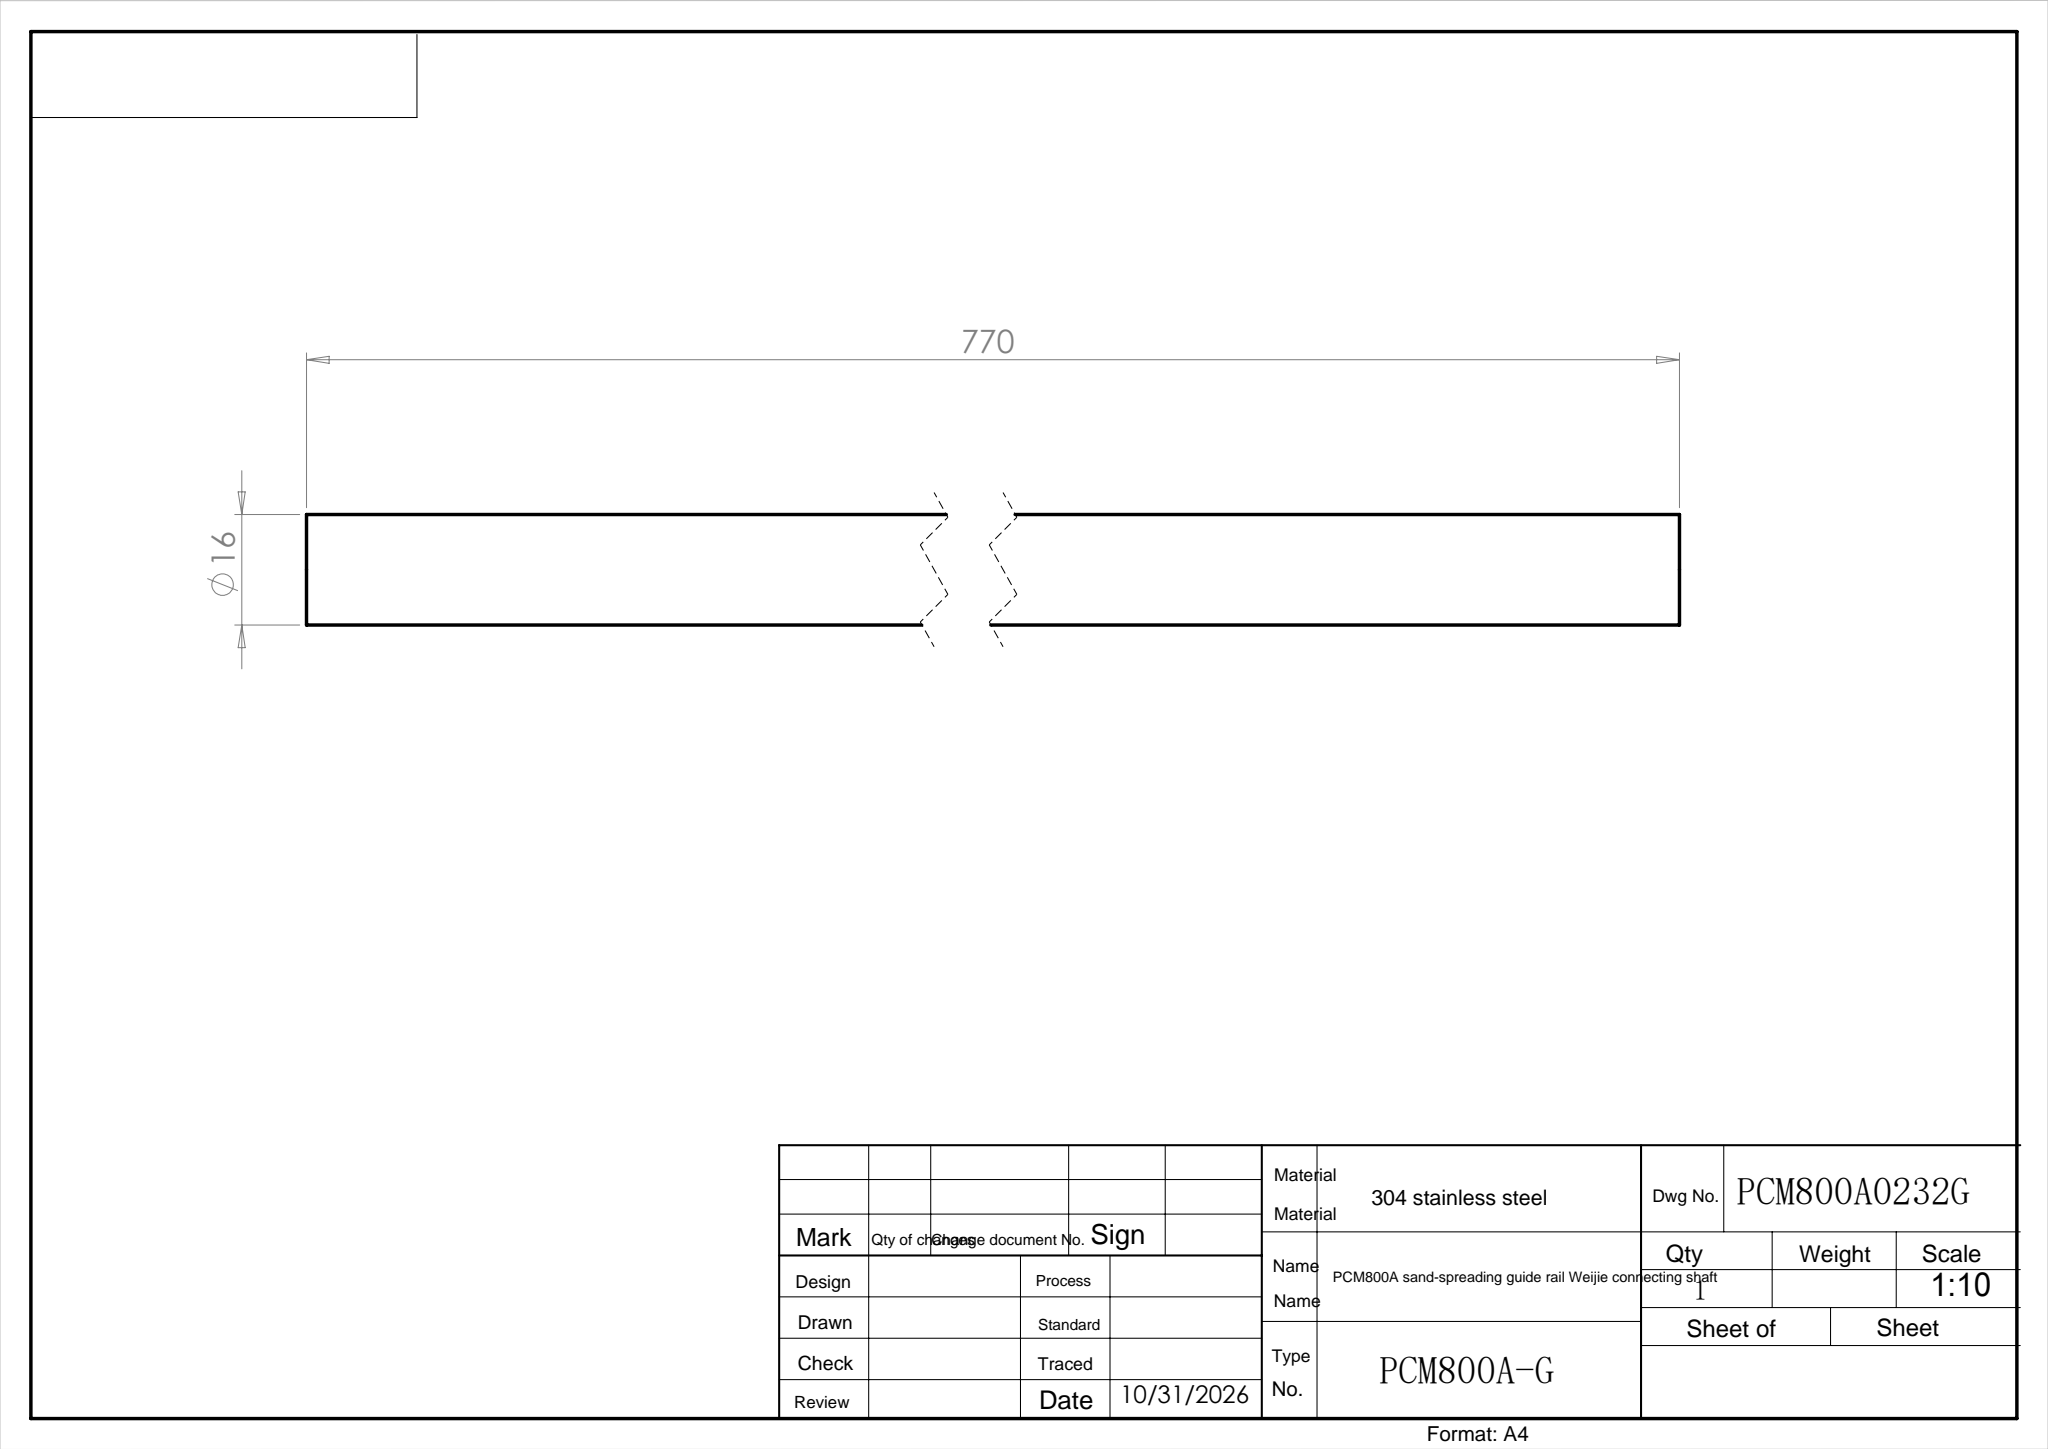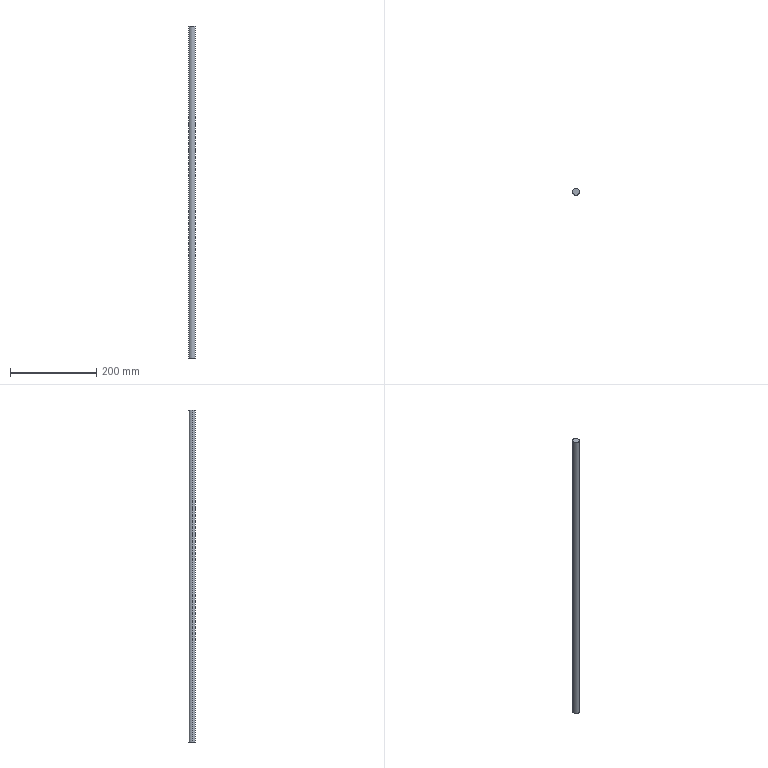Part | SolidWorks | features Extrusion 1 | 1 solid | 4 faces | box 16 x 16 x 770 mm | volume 154818 mm3 | cylinder 2 | plane 2 | commonest cylinder face diameters 16 x2
STEP:
#1=CARTESIAN_POINT('',(8.,0.,770.));
#2=VERTEX_POINT('',#1);
#3=CARTESIAN_POINT('',(-8.,0.,770.));
#4=VERTEX_POINT('',#3);
#5=CARTESIAN_POINT('',(0.,0.,770.));
#6=DIRECTION('',(0.,0.,1.));
#7=DIRECTION('',(1.,0.,0.));
#8=AXIS2_PLACEMENT_3D('',#5,#6,#7);
#9=CIRCLE('',#8,8.);
#10=EDGE_CURVE('',#2,#4,#9,.T.);
#11=ORIENTED_EDGE('',*,*,#10,.F.);
#12=CARTESIAN_POINT('',(8.,0.,0.));
#13=VERTEX_POINT('',#12);
#14=CARTESIAN_POINT('',(8.,0.,770.));
#15=DIRECTION('',(0.,0.,-1.));
#16=VECTOR('',#15,1000.);
#17=LINE('',#14,#16);
#18=EDGE_CURVE('',#2,#13,#17,.T.);
#19=ORIENTED_EDGE('',*,*,#18,.T.);
#20=CARTESIAN_POINT('',(-8.,0.,0.));
#21=VERTEX_POINT('',#20);
#22=CARTESIAN_POINT('',(0.,0.,0.));
#23=DIRECTION('',(0.,0.,1.));
#24=DIRECTION('',(1.,0.,0.));
#25=AXIS2_PLACEMENT_3D('',#22,#23,#24);
#26=CIRCLE('',#25,8.);
#27=EDGE_CURVE('',#13,#21,#26,.T.);
#28=ORIENTED_EDGE('',*,*,#27,.T.);
#29=CARTESIAN_POINT('',(-8.,0.,770.));
#30=DIRECTION('',(0.,0.,-1.));
#31=VECTOR('',#30,1000.);
#32=LINE('',#29,#31);
#33=EDGE_CURVE('',#4,#21,#32,.T.);
#34=ORIENTED_EDGE('',*,*,#33,.F.);
#35=EDGE_LOOP('',(#11,#19,#28,#34));
#36=FACE_OUTER_BOUND('',#35,.T.);
#37=CARTESIAN_POINT('',(0.,0.,770.));
#38=DIRECTION('',(0.,0.,-1.));
#39=DIRECTION('',(-1.,0.,0.));
#40=AXIS2_PLACEMENT_3D('',#37,#38,#39);
#41=CYLINDRICAL_SURFACE('',#40,8.);
#42=ADVANCED_FACE('',(#36),#41,.T.);
#43=ORIENTED_EDGE('',*,*,#18,.F.);
#44=CARTESIAN_POINT('',(0.,0.,770.));
#45=DIRECTION('',(0.,0.,1.));
#46=DIRECTION('',(1.,0.,0.));
#47=AXIS2_PLACEMENT_3D('',#44,#45,#46);
#48=CIRCLE('',#47,8.);
#49=EDGE_CURVE('',#4,#2,#48,.T.);
#50=ORIENTED_EDGE('',*,*,#49,.F.);
#51=ORIENTED_EDGE('',*,*,#33,.T.);
#52=CARTESIAN_POINT('',(0.,0.,0.));
#53=DIRECTION('',(0.,0.,1.));
#54=DIRECTION('',(1.,0.,0.));
#55=AXIS2_PLACEMENT_3D('',#52,#53,#54);
#56=CIRCLE('',#55,8.);
#57=EDGE_CURVE('',#21,#13,#56,.T.);
#58=ORIENTED_EDGE('',*,*,#57,.T.);
#59=EDGE_LOOP('',(#43,#50,#51,#58));
#60=FACE_OUTER_BOUND('',#59,.T.);
#61=CARTESIAN_POINT('',(0.,0.,770.));
#62=DIRECTION('',(0.,0.,-1.));
#63=DIRECTION('',(-1.,0.,0.));
#64=AXIS2_PLACEMENT_3D('',#61,#62,#63);
#65=CYLINDRICAL_SURFACE('',#64,8.);
#66=ADVANCED_FACE('',(#60),#65,.T.);
#67=ORIENTED_EDGE('',*,*,#49,.T.);
#68=ORIENTED_EDGE('',*,*,#10,.T.);
#69=EDGE_LOOP('',(#67,#68));
#70=FACE_OUTER_BOUND('',#69,.T.);
#71=CARTESIAN_POINT('',(0.,0.,770.));
#72=DIRECTION('',(0.,0.,1.));
#73=DIRECTION('',(1.,0.,0.));
#74=AXIS2_PLACEMENT_3D('',#71,#72,#73);
#75=PLANE('',#74);
#76=ADVANCED_FACE('',(#70),#75,.T.);
#77=ORIENTED_EDGE('',*,*,#57,.F.);
#78=ORIENTED_EDGE('',*,*,#27,.F.);
#79=EDGE_LOOP('',(#77,#78));
#80=FACE_OUTER_BOUND('',#79,.T.);
#81=CARTESIAN_POINT('',(0.,0.,0.));
#82=DIRECTION('',(0.,0.,1.));
#83=DIRECTION('',(1.,0.,0.));
#84=AXIS2_PLACEMENT_3D('',#81,#82,#83);
#85=PLANE('',#84);
#86=ADVANCED_FACE('',(#80),#85,.F.);
#87=CLOSED_SHELL('',(#42,#66,#76,#86));
#88=MANIFOLD_SOLID_BREP('',#87);
#89=CARTESIAN_POINT('',(0.,0.,0.));
#90=DIRECTION('',(0.,0.,1.));
#91=DIRECTION('',(1.,0.,0.));
#92=AXIS2_PLACEMENT_3D('',#89,#90,#91);
#93=(LENGTH_UNIT()NAMED_UNIT(*)SI_UNIT(.MILLI.,.METRE.));
#94=UNCERTAINTY_MEASURE_WITH_UNIT(LENGTH_MEASURE(0.00001),#93,'','');
#95=(NAMED_UNIT(*)PLANE_ANGLE_UNIT()SI_UNIT($,.RADIAN.));
#96=(NAMED_UNIT(*)SI_UNIT($,.STERADIAN.)SOLID_ANGLE_UNIT());
#97=(GEOMETRIC_REPRESENTATION_CONTEXT(3)GLOBAL_UNCERTAINTY_ASSIGNED_CONTEXT((#94))GLOBAL_UNIT_ASSIGNED_CONTEXT((#93,#95,#96))REPRESENTATION_CONTEXT('',''));
#98=ADVANCED_BREP_SHAPE_REPRESENTATION('',(#88,#92),#97);